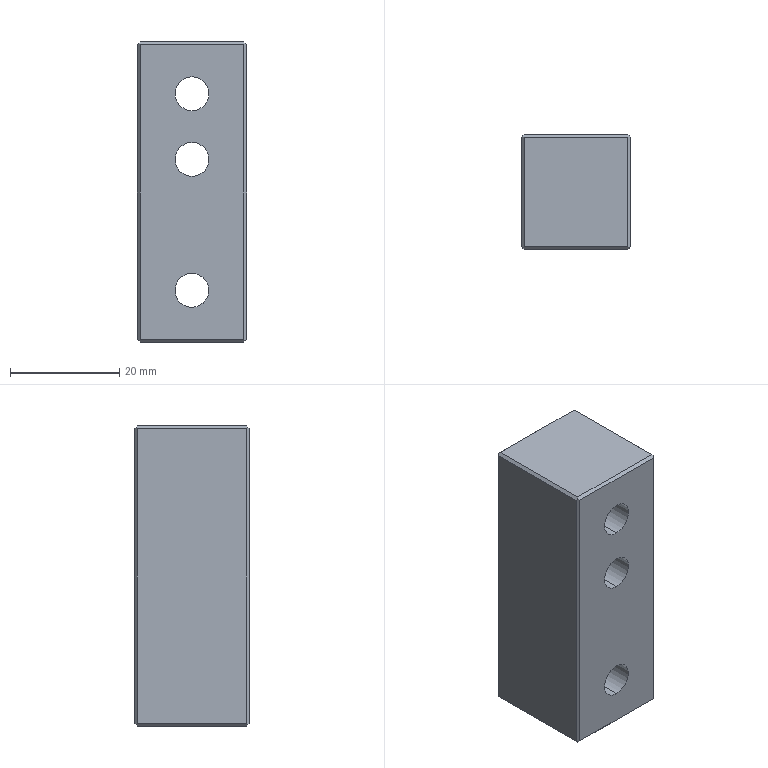Part | NX | features BREP 1 | 1 solid | 33 faces | box 20 x 21 x 55 mm | volume 20710 mm3 | plane 19 | cylinder 8 | cone 6 | commonest cylinder face diameters 6.2 x6 9.5 x2
STEP:
#1=CARTESIAN_POINT('',(0.,20.5,7.25));
#2=VERTEX_POINT('',#1);
#3=CARTESIAN_POINT('',(0.,20.5,16.75));
#4=VERTEX_POINT('',#3);
#5=CARTESIAN_POINT('',(0.,20.5,12.));
#6=DIRECTION('',(0.,1.,0.));
#7=DIRECTION('',(0.,0.,1.));
#8=AXIS2_PLACEMENT_3D('',#5,#6,#7);
#9=CIRCLE('',#8,4.75);
#10=EDGE_CURVE('',#2,#4,#9,.T.);
#11=ORIENTED_EDGE('',*,*,#10,.F.);
#12=CARTESIAN_POINT('',(0.,21.,6.75));
#13=VERTEX_POINT('',#12);
#14=CARTESIAN_POINT('',(0.,21.,6.75));
#15=DIRECTION('',(0.,0.7071,-0.7071));
#16=VECTOR('',#15,1000.);
#17=LINE('',#14,#16);
#18=EDGE_CURVE('',#2,#13,#17,.T.);
#19=ORIENTED_EDGE('',*,*,#18,.T.);
#20=CARTESIAN_POINT('',(0.,21.,17.25));
#21=VERTEX_POINT('',#20);
#22=CARTESIAN_POINT('',(0.,21.,12.));
#23=DIRECTION('',(0.,-1.,0.));
#24=DIRECTION('',(0.,0.,1.));
#25=AXIS2_PLACEMENT_3D('',#22,#23,#24);
#26=CIRCLE('',#25,5.25);
#27=EDGE_CURVE('',#21,#13,#26,.T.);
#28=ORIENTED_EDGE('',*,*,#27,.F.);
#29=CARTESIAN_POINT('',(0.,21.,17.25));
#30=DIRECTION('',(0.,0.7071,0.7071));
#31=VECTOR('',#30,1000.);
#32=LINE('',#29,#31);
#33=EDGE_CURVE('',#4,#21,#32,.T.);
#34=ORIENTED_EDGE('',*,*,#33,.F.);
#35=EDGE_LOOP('',(#11,#19,#28,#34));
#36=FACE_BOUND('',#35,.T.);
#37=CARTESIAN_POINT('',(0.,21.,12.));
#38=DIRECTION('',(0.,1.,0.));
#39=DIRECTION('',(0.,0.,-1.));
#40=AXIS2_PLACEMENT_3D('',#37,#38,#39);
#41=CONICAL_SURFACE('',#40,5.25,0.7854);
#42=ADVANCED_FACE('',(#36),#41,.F.);
#43=CARTESIAN_POINT('',(-0.02287,20.5,-27.126));
#44=VERTEX_POINT('',#43);
#45=CARTESIAN_POINT('',(-0.02287,20.5,-20.926));
#46=VERTEX_POINT('',#45);
#47=CARTESIAN_POINT('',(-0.02287,20.5,-24.026));
#48=DIRECTION('',(0.,1.,0.));
#49=DIRECTION('',(0.,0.,1.));
#50=AXIS2_PLACEMENT_3D('',#47,#48,#49);
#51=CIRCLE('',#50,3.1);
#52=EDGE_CURVE('',#44,#46,#51,.T.);
#53=ORIENTED_EDGE('',*,*,#52,.F.);
#54=CARTESIAN_POINT('',(-0.02287,21.,-27.626));
#55=VERTEX_POINT('',#54);
#56=CARTESIAN_POINT('',(-0.02287,21.,-27.626));
#57=DIRECTION('',(0.,0.7071,-0.7071));
#58=VECTOR('',#57,1000.);
#59=LINE('',#56,#58);
#60=EDGE_CURVE('',#44,#55,#59,.T.);
#61=ORIENTED_EDGE('',*,*,#60,.T.);
#62=CARTESIAN_POINT('',(-0.02287,21.,-20.426));
#63=VERTEX_POINT('',#62);
#64=CARTESIAN_POINT('',(-0.02287,21.,-24.026));
#65=DIRECTION('',(0.,-1.,0.));
#66=DIRECTION('',(0.,0.,1.));
#67=AXIS2_PLACEMENT_3D('',#64,#65,#66);
#68=CIRCLE('',#67,3.6);
#69=EDGE_CURVE('',#63,#55,#68,.T.);
#70=ORIENTED_EDGE('',*,*,#69,.F.);
#71=CARTESIAN_POINT('',(-0.02287,21.,-20.426));
#72=DIRECTION('',(0.,0.7071,0.7071));
#73=VECTOR('',#72,1000.);
#74=LINE('',#71,#73);
#75=EDGE_CURVE('',#46,#63,#74,.T.);
#76=ORIENTED_EDGE('',*,*,#75,.F.);
#77=EDGE_LOOP('',(#53,#61,#70,#76));
#78=FACE_BOUND('',#77,.T.);
#79=CARTESIAN_POINT('',(-0.02287,21.,-24.026));
#80=DIRECTION('',(0.,1.,0.));
#81=DIRECTION('',(0.,0.,-1.));
#82=AXIS2_PLACEMENT_3D('',#79,#80,#81);
#83=CONICAL_SURFACE('',#82,3.6,0.7854);
#84=ADVANCED_FACE('',(#78),#83,.F.);
#85=CARTESIAN_POINT('',(0.,20.5,-3.126));
#86=VERTEX_POINT('',#85);
#87=CARTESIAN_POINT('',(0.,20.5,3.074));
#88=VERTEX_POINT('',#87);
#89=CARTESIAN_POINT('',(0.,20.5,-0.02589));
#90=DIRECTION('',(0.,1.,0.));
#91=DIRECTION('',(0.,0.,1.));
#92=AXIS2_PLACEMENT_3D('',#89,#90,#91);
#93=CIRCLE('',#92,3.1);
#94=EDGE_CURVE('',#86,#88,#93,.T.);
#95=ORIENTED_EDGE('',*,*,#94,.F.);
#96=CARTESIAN_POINT('',(0.,21.,-3.626));
#97=VERTEX_POINT('',#96);
#98=CARTESIAN_POINT('',(0.,21.,-3.626));
#99=DIRECTION('',(0.,0.7071,-0.7071));
#100=VECTOR('',#99,1000.);
#101=LINE('',#98,#100);
#102=EDGE_CURVE('',#86,#97,#101,.T.);
#103=ORIENTED_EDGE('',*,*,#102,.T.);
#104=CARTESIAN_POINT('',(0.,21.,3.574));
#105=VERTEX_POINT('',#104);
#106=CARTESIAN_POINT('',(0.,21.,-0.02589));
#107=DIRECTION('',(0.,-1.,0.));
#108=DIRECTION('',(0.,0.,1.));
#109=AXIS2_PLACEMENT_3D('',#106,#107,#108);
#110=CIRCLE('',#109,3.6);
#111=EDGE_CURVE('',#105,#97,#110,.T.);
#112=ORIENTED_EDGE('',*,*,#111,.F.);
#113=CARTESIAN_POINT('',(0.,21.,3.574));
#114=DIRECTION('',(0.,0.7071,0.7071));
#115=VECTOR('',#114,1000.);
#116=LINE('',#113,#115);
#117=EDGE_CURVE('',#88,#105,#116,.T.);
#118=ORIENTED_EDGE('',*,*,#117,.F.);
#119=EDGE_LOOP('',(#95,#103,#112,#118));
#120=FACE_BOUND('',#119,.T.);
#121=CARTESIAN_POINT('',(0.,21.,-0.02589));
#122=DIRECTION('',(0.,1.,0.));
#123=DIRECTION('',(0.,0.,-1.));
#124=AXIS2_PLACEMENT_3D('',#121,#122,#123);
#125=CONICAL_SURFACE('',#124,3.6,0.7854);
#126=ADVANCED_FACE('',(#120),#125,.F.);
#127=CARTESIAN_POINT('',(-0.02287,0.,-20.926));
#128=VERTEX_POINT('',#127);
#129=CARTESIAN_POINT('',(-0.02287,0.,-27.126));
#130=VERTEX_POINT('',#129);
#131=CARTESIAN_POINT('',(-0.02287,0.,-24.026));
#132=DIRECTION('',(0.,-1.,0.));
#133=DIRECTION('',(0.,0.,1.));
#134=AXIS2_PLACEMENT_3D('',#131,#132,#133);
#135=CIRCLE('',#134,3.1);
#136=EDGE_CURVE('',#128,#130,#135,.T.);
#137=ORIENTED_EDGE('',*,*,#136,.T.);
#138=CARTESIAN_POINT('',(-0.02287,21.,-27.126));
#139=DIRECTION('',(0.,1.,0.));
#140=VECTOR('',#139,1000.);
#141=LINE('',#138,#140);
#142=EDGE_CURVE('',#130,#44,#141,.T.);
#143=ORIENTED_EDGE('',*,*,#142,.T.);
#144=ORIENTED_EDGE('',*,*,#52,.T.);
#145=CARTESIAN_POINT('',(-0.02287,21.,-20.926));
#146=DIRECTION('',(0.,1.,0.));
#147=VECTOR('',#146,1000.);
#148=LINE('',#145,#147);
#149=EDGE_CURVE('',#128,#46,#148,.T.);
#150=ORIENTED_EDGE('',*,*,#149,.F.);
#151=EDGE_LOOP('',(#137,#143,#144,#150));
#152=FACE_BOUND('',#151,.T.);
#153=CARTESIAN_POINT('',(-0.02287,21.,-24.026));
#154=DIRECTION('',(0.,1.,0.));
#155=DIRECTION('',(0.,0.,-1.));
#156=AXIS2_PLACEMENT_3D('',#153,#154,#155);
#157=CYLINDRICAL_SURFACE('',#156,3.1);
#158=ADVANCED_FACE('',(#152),#157,.F.);
#159=CARTESIAN_POINT('',(0.,0.,15.1));
#160=VERTEX_POINT('',#159);
#161=CARTESIAN_POINT('',(0.,0.,8.9));
#162=VERTEX_POINT('',#161);
#163=CARTESIAN_POINT('',(0.,0.,12.));
#164=DIRECTION('',(0.,-1.,0.));
#165=DIRECTION('',(0.,0.,1.));
#166=AXIS2_PLACEMENT_3D('',#163,#164,#165);
#167=CIRCLE('',#166,3.1);
#168=EDGE_CURVE('',#160,#162,#167,.T.);
#169=ORIENTED_EDGE('',*,*,#168,.T.);
#170=CARTESIAN_POINT('',(0.,10.4,8.9));
#171=VERTEX_POINT('',#170);
#172=CARTESIAN_POINT('',(0.,21.,8.9));
#173=DIRECTION('',(0.,1.,0.));
#174=VECTOR('',#173,1000.);
#175=LINE('',#172,#174);
#176=EDGE_CURVE('',#162,#171,#175,.T.);
#177=ORIENTED_EDGE('',*,*,#176,.T.);
#178=CARTESIAN_POINT('',(0.,10.4,15.1));
#179=VERTEX_POINT('',#178);
#180=CARTESIAN_POINT('',(0.,10.4,12.));
#181=DIRECTION('',(0.,-1.,0.));
#182=DIRECTION('',(0.,0.,1.));
#183=AXIS2_PLACEMENT_3D('',#180,#181,#182);
#184=CIRCLE('',#183,3.1);
#185=EDGE_CURVE('',#179,#171,#184,.T.);
#186=ORIENTED_EDGE('',*,*,#185,.F.);
#187=CARTESIAN_POINT('',(0.,21.,15.1));
#188=DIRECTION('',(0.,1.,0.));
#189=VECTOR('',#188,1000.);
#190=LINE('',#187,#189);
#191=EDGE_CURVE('',#160,#179,#190,.T.);
#192=ORIENTED_EDGE('',*,*,#191,.F.);
#193=EDGE_LOOP('',(#169,#177,#186,#192));
#194=FACE_BOUND('',#193,.T.);
#195=CARTESIAN_POINT('',(0.,21.,12.));
#196=DIRECTION('',(0.,1.,0.));
#197=DIRECTION('',(0.,0.,-1.));
#198=AXIS2_PLACEMENT_3D('',#195,#196,#197);
#199=CYLINDRICAL_SURFACE('',#198,3.1);
#200=ADVANCED_FACE('',(#194),#199,.F.);
#201=CARTESIAN_POINT('',(0.,0.,3.074));
#202=VERTEX_POINT('',#201);
#203=CARTESIAN_POINT('',(0.,0.,-3.126));
#204=VERTEX_POINT('',#203);
#205=CARTESIAN_POINT('',(0.,0.,-0.02589));
#206=DIRECTION('',(0.,-1.,0.));
#207=DIRECTION('',(0.,0.,1.));
#208=AXIS2_PLACEMENT_3D('',#205,#206,#207);
#209=CIRCLE('',#208,3.1);
#210=EDGE_CURVE('',#202,#204,#209,.T.);
#211=ORIENTED_EDGE('',*,*,#210,.T.);
#212=CARTESIAN_POINT('',(0.,21.,-3.126));
#213=DIRECTION('',(0.,1.,0.));
#214=VECTOR('',#213,1000.);
#215=LINE('',#212,#214);
#216=EDGE_CURVE('',#204,#86,#215,.T.);
#217=ORIENTED_EDGE('',*,*,#216,.T.);
#218=ORIENTED_EDGE('',*,*,#94,.T.);
#219=CARTESIAN_POINT('',(0.,21.,3.074));
#220=DIRECTION('',(0.,1.,0.));
#221=VECTOR('',#220,1000.);
#222=LINE('',#219,#221);
#223=EDGE_CURVE('',#202,#88,#222,.T.);
#224=ORIENTED_EDGE('',*,*,#223,.F.);
#225=EDGE_LOOP('',(#211,#217,#218,#224));
#226=FACE_BOUND('',#225,.T.);
#227=CARTESIAN_POINT('',(0.,21.,-0.02589));
#228=DIRECTION('',(0.,1.,0.));
#229=DIRECTION('',(0.,0.,-1.));
#230=AXIS2_PLACEMENT_3D('',#227,#228,#229);
#231=CYLINDRICAL_SURFACE('',#230,3.1);
#232=ADVANCED_FACE('',(#226),#231,.F.);
#233=CARTESIAN_POINT('',(0.,10.4,7.25));
#234=VERTEX_POINT('',#233);
#235=CARTESIAN_POINT('',(0.,10.4,16.75));
#236=VERTEX_POINT('',#235);
#237=CARTESIAN_POINT('',(0.,10.4,12.));
#238=DIRECTION('',(0.,1.,0.));
#239=DIRECTION('',(0.,0.,1.));
#240=AXIS2_PLACEMENT_3D('',#237,#238,#239);
#241=CIRCLE('',#240,4.75);
#242=EDGE_CURVE('',#234,#236,#241,.T.);
#243=ORIENTED_EDGE('',*,*,#242,.F.);
#244=CARTESIAN_POINT('',(0.,21.,7.25));
#245=DIRECTION('',(0.,1.,0.));
#246=VECTOR('',#245,1000.);
#247=LINE('',#244,#246);
#248=EDGE_CURVE('',#234,#2,#247,.T.);
#249=ORIENTED_EDGE('',*,*,#248,.T.);
#250=ORIENTED_EDGE('',*,*,#10,.T.);
#251=CARTESIAN_POINT('',(0.,21.,16.75));
#252=DIRECTION('',(0.,1.,0.));
#253=VECTOR('',#252,1000.);
#254=LINE('',#251,#253);
#255=EDGE_CURVE('',#236,#4,#254,.T.);
#256=ORIENTED_EDGE('',*,*,#255,.F.);
#257=EDGE_LOOP('',(#243,#249,#250,#256));
#258=FACE_BOUND('',#257,.T.);
#259=CARTESIAN_POINT('',(0.,21.,12.));
#260=DIRECTION('',(0.,1.,0.));
#261=DIRECTION('',(0.,0.,-1.));
#262=AXIS2_PLACEMENT_3D('',#259,#260,#261);
#263=CYLINDRICAL_SURFACE('',#262,4.75);
#264=ADVANCED_FACE('',(#258),#263,.F.);
#265=CARTESIAN_POINT('',(10.,0.5,-33.));
#266=VERTEX_POINT('',#265);
#267=CARTESIAN_POINT('',(10.,20.5,-33.));
#268=VERTEX_POINT('',#267);
#269=CARTESIAN_POINT('',(10.,0.,-33.));
#270=DIRECTION('',(0.,1.,0.));
#271=VECTOR('',#270,1000.);
#272=LINE('',#269,#271);
#273=EDGE_CURVE('',#266,#268,#272,.T.);
#274=ORIENTED_EDGE('',*,*,#273,.T.);
#275=CARTESIAN_POINT('',(10.,20.5,21.));
#276=VERTEX_POINT('',#275);
#277=CARTESIAN_POINT('',(10.,20.5,36.5));
#278=DIRECTION('',(0.,0.,1.));
#279=VECTOR('',#278,1000.);
#280=LINE('',#277,#279);
#281=EDGE_CURVE('',#268,#276,#280,.T.);
#282=ORIENTED_EDGE('',*,*,#281,.T.);
#283=CARTESIAN_POINT('',(10.,0.5,21.));
#284=VERTEX_POINT('',#283);
#285=CARTESIAN_POINT('',(10.,0.,21.));
#286=DIRECTION('',(0.,-1.,0.));
#287=VECTOR('',#286,1000.);
#288=LINE('',#285,#287);
#289=EDGE_CURVE('',#276,#284,#288,.T.);
#290=ORIENTED_EDGE('',*,*,#289,.T.);
#291=CARTESIAN_POINT('',(10.,0.5,36.5));
#292=DIRECTION('',(0.,0.,-1.));
#293=VECTOR('',#292,1000.);
#294=LINE('',#291,#293);
#295=EDGE_CURVE('',#284,#266,#294,.T.);
#296=ORIENTED_EDGE('',*,*,#295,.T.);
#297=EDGE_LOOP('',(#274,#282,#290,#296));
#298=FACE_BOUND('',#297,.T.);
#299=CARTESIAN_POINT('',(10.,0.,36.5));
#300=DIRECTION('',(1.,0.,0.));
#301=DIRECTION('',(0.,0.,1.));
#302=AXIS2_PLACEMENT_3D('',#299,#300,#301);
#303=PLANE('',#302);
#304=ADVANCED_FACE('',(#298),#303,.T.);
#305=CARTESIAN_POINT('',(9.5,21.,-33.));
#306=VERTEX_POINT('',#305);
#307=CARTESIAN_POINT('',(9.5,21.,21.));
#308=VERTEX_POINT('',#307);
#309=CARTESIAN_POINT('',(9.5,21.,-6.));
#310=DIRECTION('',(0.,0.,1.));
#311=VECTOR('',#310,1000.);
#312=LINE('',#309,#311);
#313=EDGE_CURVE('',#306,#308,#312,.T.);
#314=ORIENTED_EDGE('',*,*,#313,.T.);
#315=CARTESIAN_POINT('',(9.75,20.75,21.25));
#316=VERTEX_POINT('',#315);
#317=CARTESIAN_POINT('',(9.75,20.75,21.25));
#318=DIRECTION('',(-0.5774,0.5774,-0.5774));
#319=VECTOR('',#318,1000.);
#320=LINE('',#317,#319);
#321=EDGE_CURVE('',#316,#308,#320,.T.);
#322=ORIENTED_EDGE('',*,*,#321,.F.);
#323=CARTESIAN_POINT('',(9.75,20.75,21.25));
#324=DIRECTION('',(0.5774,-0.5774,-0.5774));
#325=VECTOR('',#324,1000.);
#326=LINE('',#323,#325);
#327=EDGE_CURVE('',#316,#276,#326,.T.);
#328=ORIENTED_EDGE('',*,*,#327,.T.);
#329=ORIENTED_EDGE('',*,*,#281,.F.);
#330=CARTESIAN_POINT('',(9.75,20.75,-33.25));
#331=VERTEX_POINT('',#330);
#332=CARTESIAN_POINT('',(10.,20.5,-33.));
#333=DIRECTION('',(-0.5774,0.5774,-0.5774));
#334=VECTOR('',#333,1000.);
#335=LINE('',#332,#334);
#336=EDGE_CURVE('',#268,#331,#335,.T.);
#337=ORIENTED_EDGE('',*,*,#336,.T.);
#338=CARTESIAN_POINT('',(9.5,21.,-33.));
#339=DIRECTION('',(0.5774,-0.5774,-0.5774));
#340=VECTOR('',#339,1000.);
#341=LINE('',#338,#340);
#342=EDGE_CURVE('',#306,#331,#341,.T.);
#343=ORIENTED_EDGE('',*,*,#342,.F.);
#344=EDGE_LOOP('',(#314,#322,#328,#329,#337,#343));
#345=FACE_BOUND('',#344,.T.);
#346=CARTESIAN_POINT('',(9.75,20.75,-6.));
#347=DIRECTION('',(0.7071,0.7071,0.));
#348=DIRECTION('',(0.7071,-0.7071,0.));
#349=AXIS2_PLACEMENT_3D('',#346,#347,#348);
#350=PLANE('',#349);
#351=ADVANCED_FACE('',(#345),#350,.T.);
#352=ORIENTED_EDGE('',*,*,#273,.F.);
#353=CARTESIAN_POINT('',(9.75,0.25,-33.25));
#354=VERTEX_POINT('',#353);
#355=CARTESIAN_POINT('',(10.,0.5,-33.));
#356=DIRECTION('',(-0.5774,-0.5774,-0.5774));
#357=VECTOR('',#356,1000.);
#358=LINE('',#355,#357);
#359=EDGE_CURVE('',#266,#354,#358,.T.);
#360=ORIENTED_EDGE('',*,*,#359,.T.);
#361=CARTESIAN_POINT('',(9.5,0.5,-33.5));
#362=VERTEX_POINT('',#361);
#363=CARTESIAN_POINT('',(9.5,0.5,-33.5));
#364=DIRECTION('',(0.5774,-0.5774,0.5774));
#365=VECTOR('',#364,1000.);
#366=LINE('',#363,#365);
#367=EDGE_CURVE('',#362,#354,#366,.T.);
#368=ORIENTED_EDGE('',*,*,#367,.F.);
#369=CARTESIAN_POINT('',(9.5,20.5,-33.5));
#370=VERTEX_POINT('',#369);
#371=CARTESIAN_POINT('',(9.5,10.5,-33.5));
#372=DIRECTION('',(0.,1.,0.));
#373=VECTOR('',#372,1000.);
#374=LINE('',#371,#373);
#375=EDGE_CURVE('',#362,#370,#374,.T.);
#376=ORIENTED_EDGE('',*,*,#375,.T.);
#377=CARTESIAN_POINT('',(9.75,20.75,-33.25));
#378=DIRECTION('',(-0.5774,-0.5774,-0.5774));
#379=VECTOR('',#378,1000.);
#380=LINE('',#377,#379);
#381=EDGE_CURVE('',#331,#370,#380,.T.);
#382=ORIENTED_EDGE('',*,*,#381,.F.);
#383=ORIENTED_EDGE('',*,*,#336,.F.);
#384=EDGE_LOOP('',(#352,#360,#368,#376,#382,#383));
#385=FACE_BOUND('',#384,.T.);
#386=CARTESIAN_POINT('',(9.75,10.5,-33.25));
#387=DIRECTION('',(0.7071,0.,-0.7071));
#388=DIRECTION('',(0.7071,0.,0.7071));
#389=AXIS2_PLACEMENT_3D('',#386,#387,#388);
#390=PLANE('',#389);
#391=ADVANCED_FACE('',(#385),#390,.T.);
#392=ORIENTED_EDGE('',*,*,#295,.F.);
#393=CARTESIAN_POINT('',(9.75,0.25,21.25));
#394=VERTEX_POINT('',#393);
#395=CARTESIAN_POINT('',(10.,0.5,21.));
#396=DIRECTION('',(-0.5774,-0.5774,0.5774));
#397=VECTOR('',#396,1000.);
#398=LINE('',#395,#397);
#399=EDGE_CURVE('',#284,#394,#398,.T.);
#400=ORIENTED_EDGE('',*,*,#399,.T.);
#401=CARTESIAN_POINT('',(9.5,0.,21.));
#402=VERTEX_POINT('',#401);
#403=CARTESIAN_POINT('',(9.5,0.,21.));
#404=DIRECTION('',(0.5774,0.5774,0.5774));
#405=VECTOR('',#404,1000.);
#406=LINE('',#403,#405);
#407=EDGE_CURVE('',#402,#394,#406,.T.);
#408=ORIENTED_EDGE('',*,*,#407,.F.);
#409=CARTESIAN_POINT('',(9.5,0.,-33.));
#410=VERTEX_POINT('',#409);
#411=CARTESIAN_POINT('',(9.5,0.,-6.));
#412=DIRECTION('',(0.,0.,-1.));
#413=VECTOR('',#412,1000.);
#414=LINE('',#411,#413);
#415=EDGE_CURVE('',#402,#410,#414,.T.);
#416=ORIENTED_EDGE('',*,*,#415,.T.);
#417=CARTESIAN_POINT('',(9.75,0.25,-33.25));
#418=DIRECTION('',(-0.5774,-0.5774,0.5774));
#419=VECTOR('',#418,1000.);
#420=LINE('',#417,#419);
#421=EDGE_CURVE('',#354,#410,#420,.T.);
#422=ORIENTED_EDGE('',*,*,#421,.F.);
#423=ORIENTED_EDGE('',*,*,#359,.F.);
#424=EDGE_LOOP('',(#392,#400,#408,#416,#422,#423));
#425=FACE_BOUND('',#424,.T.);
#426=CARTESIAN_POINT('',(9.75,0.25,-6.));
#427=DIRECTION('',(0.7071,-0.7071,0.));
#428=DIRECTION('',(-0.7071,-0.7071,0.));
#429=AXIS2_PLACEMENT_3D('',#426,#427,#428);
#430=PLANE('',#429);
#431=ADVANCED_FACE('',(#425),#430,.T.);
#432=CARTESIAN_POINT('',(9.5,20.5,21.5));
#433=VERTEX_POINT('',#432);
#434=CARTESIAN_POINT('',(9.5,0.5,21.5));
#435=VERTEX_POINT('',#434);
#436=CARTESIAN_POINT('',(9.5,10.5,21.5));
#437=DIRECTION('',(0.,-1.,0.));
#438=VECTOR('',#437,1000.);
#439=LINE('',#436,#438);
#440=EDGE_CURVE('',#433,#435,#439,.T.);
#441=ORIENTED_EDGE('',*,*,#440,.T.);
#442=CARTESIAN_POINT('',(9.75,0.25,21.25));
#443=DIRECTION('',(-0.5774,0.5774,0.5774));
#444=VECTOR('',#443,1000.);
#445=LINE('',#442,#444);
#446=EDGE_CURVE('',#394,#435,#445,.T.);
#447=ORIENTED_EDGE('',*,*,#446,.F.);
#448=ORIENTED_EDGE('',*,*,#399,.F.);
#449=ORIENTED_EDGE('',*,*,#289,.F.);
#450=ORIENTED_EDGE('',*,*,#327,.F.);
#451=CARTESIAN_POINT('',(9.5,20.5,21.5));
#452=DIRECTION('',(0.5774,0.5774,-0.5774));
#453=VECTOR('',#452,1000.);
#454=LINE('',#451,#453);
#455=EDGE_CURVE('',#433,#316,#454,.T.);
#456=ORIENTED_EDGE('',*,*,#455,.F.);
#457=EDGE_LOOP('',(#441,#447,#448,#449,#450,#456));
#458=FACE_BOUND('',#457,.T.);
#459=CARTESIAN_POINT('',(9.75,10.5,21.25));
#460=DIRECTION('',(0.7071,0.,0.7071));
#461=DIRECTION('',(-0.7071,0.,0.7071));
#462=AXIS2_PLACEMENT_3D('',#459,#460,#461);
#463=PLANE('',#462);
#464=ADVANCED_FACE('',(#458),#463,.T.);
#465=CARTESIAN_POINT('',(-9.5,21.,21.));
#466=VERTEX_POINT('',#465);
#467=CARTESIAN_POINT('',(0.,21.,21.));
#468=DIRECTION('',(1.,0.,0.));
#469=VECTOR('',#468,1000.);
#470=LINE('',#467,#469);
#471=EDGE_CURVE('',#466,#308,#470,.T.);
#472=ORIENTED_EDGE('',*,*,#471,.T.);
#473=ORIENTED_EDGE('',*,*,#313,.F.);
#474=CARTESIAN_POINT('',(-9.5,21.,-33.));
#475=VERTEX_POINT('',#474);
#476=CARTESIAN_POINT('',(0.,21.,-33.));
#477=DIRECTION('',(-1.,0.,0.));
#478=VECTOR('',#477,1000.);
#479=LINE('',#476,#478);
#480=EDGE_CURVE('',#306,#475,#479,.T.);
#481=ORIENTED_EDGE('',*,*,#480,.T.);
#482=CARTESIAN_POINT('',(-9.5,21.,0.));
#483=DIRECTION('',(0.,0.,1.));
#484=VECTOR('',#483,1000.);
#485=LINE('',#482,#484);
#486=EDGE_CURVE('',#475,#466,#485,.T.);
#487=ORIENTED_EDGE('',*,*,#486,.T.);
#488=EDGE_LOOP('',(#472,#473,#481,#487));
#489=FACE_BOUND('',#488,.T.);
#490=ORIENTED_EDGE('',*,*,#27,.T.);
#491=CARTESIAN_POINT('',(0.,21.,12.));
#492=DIRECTION('',(0.,-1.,0.));
#493=DIRECTION('',(0.,0.,1.));
#494=AXIS2_PLACEMENT_3D('',#491,#492,#493);
#495=CIRCLE('',#494,5.25);
#496=EDGE_CURVE('',#13,#21,#495,.T.);
#497=ORIENTED_EDGE('',*,*,#496,.T.);
#498=EDGE_LOOP('',(#490,#497));
#499=FACE_BOUND('',#498,.T.);
#500=ORIENTED_EDGE('',*,*,#69,.T.);
#501=CARTESIAN_POINT('',(-0.02287,21.,-24.026));
#502=DIRECTION('',(0.,-1.,0.));
#503=DIRECTION('',(0.,0.,1.));
#504=AXIS2_PLACEMENT_3D('',#501,#502,#503);
#505=CIRCLE('',#504,3.6);
#506=EDGE_CURVE('',#55,#63,#505,.T.);
#507=ORIENTED_EDGE('',*,*,#506,.T.);
#508=EDGE_LOOP('',(#500,#507));
#509=FACE_BOUND('',#508,.T.);
#510=ORIENTED_EDGE('',*,*,#111,.T.);
#511=CARTESIAN_POINT('',(0.,21.,-0.02589));
#512=DIRECTION('',(0.,-1.,0.));
#513=DIRECTION('',(0.,0.,1.));
#514=AXIS2_PLACEMENT_3D('',#511,#512,#513);
#515=CIRCLE('',#514,3.6);
#516=EDGE_CURVE('',#97,#105,#515,.T.);
#517=ORIENTED_EDGE('',*,*,#516,.T.);
#518=EDGE_LOOP('',(#510,#517));
#519=FACE_BOUND('',#518,.T.);
#520=CARTESIAN_POINT('',(0.,21.,0.));
#521=DIRECTION('',(0.,1.,0.));
#522=DIRECTION('',(0.,0.,-1.));
#523=AXIS2_PLACEMENT_3D('',#520,#521,#522);
#524=PLANE('',#523);
#525=ADVANCED_FACE('',(#489,#499,#509,#519),#524,.T.);
#526=ORIENTED_EDGE('',*,*,#375,.F.);
#527=CARTESIAN_POINT('',(-9.5,0.5,-33.5));
#528=VERTEX_POINT('',#527);
#529=CARTESIAN_POINT('',(10.,0.5,-33.5));
#530=DIRECTION('',(-1.,0.,0.));
#531=VECTOR('',#530,1000.);
#532=LINE('',#529,#531);
#533=EDGE_CURVE('',#362,#528,#532,.T.);
#534=ORIENTED_EDGE('',*,*,#533,.T.);
#535=CARTESIAN_POINT('',(-9.5,20.5,-33.5));
#536=VERTEX_POINT('',#535);
#537=CARTESIAN_POINT('',(-9.5,0.,-33.5));
#538=DIRECTION('',(0.,1.,0.));
#539=VECTOR('',#538,1000.);
#540=LINE('',#537,#539);
#541=EDGE_CURVE('',#528,#536,#540,.T.);
#542=ORIENTED_EDGE('',*,*,#541,.T.);
#543=CARTESIAN_POINT('',(10.,20.5,-33.5));
#544=DIRECTION('',(1.,0.,0.));
#545=VECTOR('',#544,1000.);
#546=LINE('',#543,#545);
#547=EDGE_CURVE('',#536,#370,#546,.T.);
#548=ORIENTED_EDGE('',*,*,#547,.T.);
#549=EDGE_LOOP('',(#526,#534,#542,#548));
#550=FACE_BOUND('',#549,.T.);
#551=CARTESIAN_POINT('',(10.,0.,-33.5));
#552=DIRECTION('',(0.,0.,-1.));
#553=DIRECTION('',(1.,0.,0.));
#554=AXIS2_PLACEMENT_3D('',#551,#552,#553);
#555=PLANE('',#554);
#556=ADVANCED_FACE('',(#550),#555,.T.);
#557=CARTESIAN_POINT('',(-9.5,0.,-33.));
#558=VERTEX_POINT('',#557);
#559=CARTESIAN_POINT('',(0.,0.,-33.));
#560=DIRECTION('',(-1.,0.,0.));
#561=VECTOR('',#560,1000.);
#562=LINE('',#559,#561);
#563=EDGE_CURVE('',#410,#558,#562,.T.);
#564=ORIENTED_EDGE('',*,*,#563,.F.);
#565=ORIENTED_EDGE('',*,*,#415,.F.);
#566=CARTESIAN_POINT('',(-9.5,0.,21.));
#567=VERTEX_POINT('',#566);
#568=CARTESIAN_POINT('',(0.,0.,21.));
#569=DIRECTION('',(1.,0.,0.));
#570=VECTOR('',#569,1000.);
#571=LINE('',#568,#570);
#572=EDGE_CURVE('',#567,#402,#571,.T.);
#573=ORIENTED_EDGE('',*,*,#572,.F.);
#574=CARTESIAN_POINT('',(-9.5,0.,0.));
#575=DIRECTION('',(0.,0.,1.));
#576=VECTOR('',#575,1000.);
#577=LINE('',#574,#576);
#578=EDGE_CURVE('',#558,#567,#577,.T.);
#579=ORIENTED_EDGE('',*,*,#578,.F.);
#580=EDGE_LOOP('',(#564,#565,#573,#579));
#581=FACE_BOUND('',#580,.T.);
#582=ORIENTED_EDGE('',*,*,#136,.F.);
#583=CARTESIAN_POINT('',(-0.02287,0.,-24.026));
#584=DIRECTION('',(0.,-1.,0.));
#585=DIRECTION('',(0.,0.,1.));
#586=AXIS2_PLACEMENT_3D('',#583,#584,#585);
#587=CIRCLE('',#586,3.1);
#588=EDGE_CURVE('',#130,#128,#587,.T.);
#589=ORIENTED_EDGE('',*,*,#588,.F.);
#590=EDGE_LOOP('',(#582,#589));
#591=FACE_BOUND('',#590,.T.);
#592=ORIENTED_EDGE('',*,*,#168,.F.);
#593=CARTESIAN_POINT('',(0.,0.,12.));
#594=DIRECTION('',(0.,-1.,0.));
#595=DIRECTION('',(0.,0.,1.));
#596=AXIS2_PLACEMENT_3D('',#593,#594,#595);
#597=CIRCLE('',#596,3.1);
#598=EDGE_CURVE('',#162,#160,#597,.T.);
#599=ORIENTED_EDGE('',*,*,#598,.F.);
#600=EDGE_LOOP('',(#592,#599));
#601=FACE_BOUND('',#600,.T.);
#602=ORIENTED_EDGE('',*,*,#210,.F.);
#603=CARTESIAN_POINT('',(0.,0.,-0.02589));
#604=DIRECTION('',(0.,-1.,0.));
#605=DIRECTION('',(0.,0.,1.));
#606=AXIS2_PLACEMENT_3D('',#603,#604,#605);
#607=CIRCLE('',#606,3.1);
#608=EDGE_CURVE('',#204,#202,#607,.T.);
#609=ORIENTED_EDGE('',*,*,#608,.F.);
#610=EDGE_LOOP('',(#602,#609));
#611=FACE_BOUND('',#610,.T.);
#612=CARTESIAN_POINT('',(0.,0.,0.));
#613=DIRECTION('',(0.,1.,0.));
#614=DIRECTION('',(0.,0.,-1.));
#615=AXIS2_PLACEMENT_3D('',#612,#613,#614);
#616=PLANE('',#615);
#617=ADVANCED_FACE('',(#581,#591,#601,#611),#616,.F.);
#618=CARTESIAN_POINT('',(-9.5,20.5,21.5));
#619=VERTEX_POINT('',#618);
#620=CARTESIAN_POINT('',(-10.,20.5,21.5));
#621=DIRECTION('',(-1.,0.,0.));
#622=VECTOR('',#621,1000.);
#623=LINE('',#620,#622);
#624=EDGE_CURVE('',#433,#619,#623,.T.);
#625=ORIENTED_EDGE('',*,*,#624,.T.);
#626=CARTESIAN_POINT('',(-9.5,0.5,21.5));
#627=VERTEX_POINT('',#626);
#628=CARTESIAN_POINT('',(-9.5,0.,21.5));
#629=DIRECTION('',(0.,-1.,0.));
#630=VECTOR('',#629,1000.);
#631=LINE('',#628,#630);
#632=EDGE_CURVE('',#619,#627,#631,.T.);
#633=ORIENTED_EDGE('',*,*,#632,.T.);
#634=CARTESIAN_POINT('',(-10.,0.5,21.5));
#635=DIRECTION('',(1.,0.,0.));
#636=VECTOR('',#635,1000.);
#637=LINE('',#634,#636);
#638=EDGE_CURVE('',#627,#435,#637,.T.);
#639=ORIENTED_EDGE('',*,*,#638,.T.);
#640=ORIENTED_EDGE('',*,*,#440,.F.);
#641=EDGE_LOOP('',(#625,#633,#639,#640));
#642=FACE_BOUND('',#641,.T.);
#643=CARTESIAN_POINT('',(-10.,0.,21.5));
#644=DIRECTION('',(0.,0.,1.));
#645=DIRECTION('',(-1.,0.,0.));
#646=AXIS2_PLACEMENT_3D('',#643,#644,#645);
#647=PLANE('',#646);
#648=ADVANCED_FACE('',(#642),#647,.T.);
#649=ORIENTED_EDGE('',*,*,#471,.F.);
#650=CARTESIAN_POINT('',(-9.75,20.75,21.25));
#651=VERTEX_POINT('',#650);
#652=CARTESIAN_POINT('',(-9.5,21.,21.));
#653=DIRECTION('',(-0.5774,-0.5774,0.5774));
#654=VECTOR('',#653,1000.);
#655=LINE('',#652,#654);
#656=EDGE_CURVE('',#466,#651,#655,.T.);
#657=ORIENTED_EDGE('',*,*,#656,.T.);
#658=CARTESIAN_POINT('',(-9.75,20.75,21.25));
#659=DIRECTION('',(0.5774,-0.5774,0.5774));
#660=VECTOR('',#659,1000.);
#661=LINE('',#658,#660);
#662=EDGE_CURVE('',#651,#619,#661,.T.);
#663=ORIENTED_EDGE('',*,*,#662,.T.);
#664=ORIENTED_EDGE('',*,*,#624,.F.);
#665=ORIENTED_EDGE('',*,*,#455,.T.);
#666=ORIENTED_EDGE('',*,*,#321,.T.);
#667=EDGE_LOOP('',(#649,#657,#663,#664,#665,#666));
#668=FACE_BOUND('',#667,.T.);
#669=CARTESIAN_POINT('',(0.,20.75,21.25));
#670=DIRECTION('',(0.,0.7071,0.7071));
#671=DIRECTION('',(0.,0.7071,-0.7071));
#672=AXIS2_PLACEMENT_3D('',#669,#670,#671);
#673=PLANE('',#672);
#674=ADVANCED_FACE('',(#668),#673,.T.);
#675=ORIENTED_EDGE('',*,*,#486,.F.);
#676=CARTESIAN_POINT('',(-9.75,20.75,-33.25));
#677=VERTEX_POINT('',#676);
#678=CARTESIAN_POINT('',(-9.5,21.,-33.));
#679=DIRECTION('',(-0.5774,-0.5774,-0.5774));
#680=VECTOR('',#679,1000.);
#681=LINE('',#678,#680);
#682=EDGE_CURVE('',#475,#677,#681,.T.);
#683=ORIENTED_EDGE('',*,*,#682,.T.);
#684=CARTESIAN_POINT('',(-10.,20.5,-33.));
#685=VERTEX_POINT('',#684);
#686=CARTESIAN_POINT('',(-9.75,20.75,-33.25));
#687=DIRECTION('',(-0.5774,-0.5774,0.5774));
#688=VECTOR('',#687,1000.);
#689=LINE('',#686,#688);
#690=EDGE_CURVE('',#677,#685,#689,.T.);
#691=ORIENTED_EDGE('',*,*,#690,.T.);
#692=CARTESIAN_POINT('',(-10.,20.5,21.));
#693=VERTEX_POINT('',#692);
#694=CARTESIAN_POINT('',(-10.,20.5,-6.));
#695=DIRECTION('',(0.,0.,1.));
#696=VECTOR('',#695,1000.);
#697=LINE('',#694,#696);
#698=EDGE_CURVE('',#685,#693,#697,.T.);
#699=ORIENTED_EDGE('',*,*,#698,.T.);
#700=CARTESIAN_POINT('',(-10.,20.5,21.));
#701=DIRECTION('',(0.5774,0.5774,0.5774));
#702=VECTOR('',#701,1000.);
#703=LINE('',#700,#702);
#704=EDGE_CURVE('',#693,#651,#703,.T.);
#705=ORIENTED_EDGE('',*,*,#704,.T.);
#706=ORIENTED_EDGE('',*,*,#656,.F.);
#707=EDGE_LOOP('',(#675,#683,#691,#699,#705,#706));
#708=FACE_BOUND('',#707,.T.);
#709=CARTESIAN_POINT('',(-9.75,20.75,-6.));
#710=DIRECTION('',(-0.7071,0.7071,0.));
#711=DIRECTION('',(0.7071,0.7071,0.));
#712=AXIS2_PLACEMENT_3D('',#709,#710,#711);
#713=PLANE('',#712);
#714=ADVANCED_FACE('',(#708),#713,.T.);
#715=ORIENTED_EDGE('',*,*,#547,.F.);
#716=CARTESIAN_POINT('',(-9.5,20.5,-33.5));
#717=DIRECTION('',(-0.5774,0.5774,0.5774));
#718=VECTOR('',#717,1000.);
#719=LINE('',#716,#718);
#720=EDGE_CURVE('',#536,#677,#719,.T.);
#721=ORIENTED_EDGE('',*,*,#720,.T.);
#722=ORIENTED_EDGE('',*,*,#682,.F.);
#723=ORIENTED_EDGE('',*,*,#480,.F.);
#724=ORIENTED_EDGE('',*,*,#342,.T.);
#725=ORIENTED_EDGE('',*,*,#381,.T.);
#726=EDGE_LOOP('',(#715,#721,#722,#723,#724,#725));
#727=FACE_BOUND('',#726,.T.);
#728=CARTESIAN_POINT('',(0.,20.75,-33.25));
#729=DIRECTION('',(0.,0.7071,-0.7071));
#730=DIRECTION('',(0.,-0.7071,-0.7071));
#731=AXIS2_PLACEMENT_3D('',#728,#729,#730);
#732=PLANE('',#731);
#733=ADVANCED_FACE('',(#727),#732,.T.);
#734=ORIENTED_EDGE('',*,*,#18,.F.);
#735=CARTESIAN_POINT('',(0.,20.5,12.));
#736=DIRECTION('',(0.,1.,0.));
#737=DIRECTION('',(0.,0.,1.));
#738=AXIS2_PLACEMENT_3D('',#735,#736,#737);
#739=CIRCLE('',#738,4.75);
#740=EDGE_CURVE('',#4,#2,#739,.T.);
#741=ORIENTED_EDGE('',*,*,#740,.F.);
#742=ORIENTED_EDGE('',*,*,#33,.T.);
#743=ORIENTED_EDGE('',*,*,#496,.F.);
#744=EDGE_LOOP('',(#734,#741,#742,#743));
#745=FACE_BOUND('',#744,.T.);
#746=CARTESIAN_POINT('',(0.,21.,12.));
#747=DIRECTION('',(0.,1.,0.));
#748=DIRECTION('',(0.,0.,-1.));
#749=AXIS2_PLACEMENT_3D('',#746,#747,#748);
#750=CONICAL_SURFACE('',#749,5.25,0.7854);
#751=ADVANCED_FACE('',(#745),#750,.F.);
#752=ORIENTED_EDGE('',*,*,#60,.F.);
#753=CARTESIAN_POINT('',(-0.02287,20.5,-24.026));
#754=DIRECTION('',(0.,1.,0.));
#755=DIRECTION('',(0.,0.,1.));
#756=AXIS2_PLACEMENT_3D('',#753,#754,#755);
#757=CIRCLE('',#756,3.1);
#758=EDGE_CURVE('',#46,#44,#757,.T.);
#759=ORIENTED_EDGE('',*,*,#758,.F.);
#760=ORIENTED_EDGE('',*,*,#75,.T.);
#761=ORIENTED_EDGE('',*,*,#506,.F.);
#762=EDGE_LOOP('',(#752,#759,#760,#761));
#763=FACE_BOUND('',#762,.T.);
#764=CARTESIAN_POINT('',(-0.02287,21.,-24.026));
#765=DIRECTION('',(0.,1.,0.));
#766=DIRECTION('',(0.,0.,-1.));
#767=AXIS2_PLACEMENT_3D('',#764,#765,#766);
#768=CONICAL_SURFACE('',#767,3.6,0.7854);
#769=ADVANCED_FACE('',(#763),#768,.F.);
#770=ORIENTED_EDGE('',*,*,#102,.F.);
#771=CARTESIAN_POINT('',(0.,20.5,-0.02589));
#772=DIRECTION('',(0.,1.,0.));
#773=DIRECTION('',(0.,0.,1.));
#774=AXIS2_PLACEMENT_3D('',#771,#772,#773);
#775=CIRCLE('',#774,3.1);
#776=EDGE_CURVE('',#88,#86,#775,.T.);
#777=ORIENTED_EDGE('',*,*,#776,.F.);
#778=ORIENTED_EDGE('',*,*,#117,.T.);
#779=ORIENTED_EDGE('',*,*,#516,.F.);
#780=EDGE_LOOP('',(#770,#777,#778,#779));
#781=FACE_BOUND('',#780,.T.);
#782=CARTESIAN_POINT('',(0.,21.,-0.02589));
#783=DIRECTION('',(0.,1.,0.));
#784=DIRECTION('',(0.,0.,-1.));
#785=AXIS2_PLACEMENT_3D('',#782,#783,#784);
#786=CONICAL_SURFACE('',#785,3.6,0.7854);
#787=ADVANCED_FACE('',(#781),#786,.F.);
#788=ORIENTED_EDGE('',*,*,#563,.T.);
#789=CARTESIAN_POINT('',(-9.75,0.25,-33.25));
#790=VERTEX_POINT('',#789);
#791=CARTESIAN_POINT('',(-9.5,0.,-33.));
#792=DIRECTION('',(-0.5774,0.5774,-0.5774));
#793=VECTOR('',#792,1000.);
#794=LINE('',#791,#793);
#795=EDGE_CURVE('',#558,#790,#794,.T.);
#796=ORIENTED_EDGE('',*,*,#795,.T.);
#797=CARTESIAN_POINT('',(-9.75,0.25,-33.25));
#798=DIRECTION('',(0.5774,0.5774,-0.5774));
#799=VECTOR('',#798,1000.);
#800=LINE('',#797,#799);
#801=EDGE_CURVE('',#790,#528,#800,.T.);
#802=ORIENTED_EDGE('',*,*,#801,.T.);
#803=ORIENTED_EDGE('',*,*,#533,.F.);
#804=ORIENTED_EDGE('',*,*,#367,.T.);
#805=ORIENTED_EDGE('',*,*,#421,.T.);
#806=EDGE_LOOP('',(#788,#796,#802,#803,#804,#805));
#807=FACE_BOUND('',#806,.T.);
#808=CARTESIAN_POINT('',(0.,0.25,-33.25));
#809=DIRECTION('',(0.,-0.7071,-0.7071));
#810=DIRECTION('',(0.,-0.7071,0.7071));
#811=AXIS2_PLACEMENT_3D('',#808,#809,#810);
#812=PLANE('',#811);
#813=ADVANCED_FACE('',(#807),#812,.T.);
#814=ORIENTED_EDGE('',*,*,#541,.F.);
#815=ORIENTED_EDGE('',*,*,#801,.F.);
#816=CARTESIAN_POINT('',(-10.,0.5,-33.));
#817=VERTEX_POINT('',#816);
#818=CARTESIAN_POINT('',(-9.75,0.25,-33.25));
#819=DIRECTION('',(-0.5774,0.5774,0.5774));
#820=VECTOR('',#819,1000.);
#821=LINE('',#818,#820);
#822=EDGE_CURVE('',#790,#817,#821,.T.);
#823=ORIENTED_EDGE('',*,*,#822,.T.);
#824=CARTESIAN_POINT('',(-10.,10.5,-33.));
#825=DIRECTION('',(0.,1.,0.));
#826=VECTOR('',#825,1000.);
#827=LINE('',#824,#826);
#828=EDGE_CURVE('',#817,#685,#827,.T.);
#829=ORIENTED_EDGE('',*,*,#828,.T.);
#830=ORIENTED_EDGE('',*,*,#690,.F.);
#831=ORIENTED_EDGE('',*,*,#720,.F.);
#832=EDGE_LOOP('',(#814,#815,#823,#829,#830,#831));
#833=FACE_BOUND('',#832,.T.);
#834=CARTESIAN_POINT('',(-9.75,10.5,-33.25));
#835=DIRECTION('',(-0.7071,0.,-0.7071));
#836=DIRECTION('',(0.7071,0.,-0.7071));
#837=AXIS2_PLACEMENT_3D('',#834,#835,#836);
#838=PLANE('',#837);
#839=ADVANCED_FACE('',(#833),#838,.T.);
#840=CARTESIAN_POINT('',(-10.,0.5,21.));
#841=VERTEX_POINT('',#840);
#842=CARTESIAN_POINT('',(-10.,0.5,-6.));
#843=DIRECTION('',(0.,0.,-1.));
#844=VECTOR('',#843,1000.);
#845=LINE('',#842,#844);
#846=EDGE_CURVE('',#841,#817,#845,.T.);
#847=ORIENTED_EDGE('',*,*,#846,.T.);
#848=ORIENTED_EDGE('',*,*,#822,.F.);
#849=ORIENTED_EDGE('',*,*,#795,.F.);
#850=ORIENTED_EDGE('',*,*,#578,.T.);
#851=CARTESIAN_POINT('',(-9.75,0.25,21.25));
#852=VERTEX_POINT('',#851);
#853=CARTESIAN_POINT('',(-9.5,0.,21.));
#854=DIRECTION('',(-0.5774,0.5774,0.5774));
#855=VECTOR('',#854,1000.);
#856=LINE('',#853,#855);
#857=EDGE_CURVE('',#567,#852,#856,.T.);
#858=ORIENTED_EDGE('',*,*,#857,.T.);
#859=CARTESIAN_POINT('',(-9.75,0.25,21.25));
#860=DIRECTION('',(-0.5774,0.5774,-0.5774));
#861=VECTOR('',#860,1000.);
#862=LINE('',#859,#861);
#863=EDGE_CURVE('',#852,#841,#862,.T.);
#864=ORIENTED_EDGE('',*,*,#863,.T.);
#865=EDGE_LOOP('',(#847,#848,#849,#850,#858,#864));
#866=FACE_BOUND('',#865,.T.);
#867=CARTESIAN_POINT('',(-9.75,0.25,-6.));
#868=DIRECTION('',(-0.7071,-0.7071,0.));
#869=DIRECTION('',(-0.7071,0.7071,0.));
#870=AXIS2_PLACEMENT_3D('',#867,#868,#869);
#871=PLANE('',#870);
#872=ADVANCED_FACE('',(#866),#871,.T.);
#873=ORIENTED_EDGE('',*,*,#638,.F.);
#874=CARTESIAN_POINT('',(-9.5,0.5,21.5));
#875=DIRECTION('',(-0.5774,-0.5774,-0.5774));
#876=VECTOR('',#875,1000.);
#877=LINE('',#874,#876);
#878=EDGE_CURVE('',#627,#852,#877,.T.);
#879=ORIENTED_EDGE('',*,*,#878,.T.);
#880=ORIENTED_EDGE('',*,*,#857,.F.);
#881=ORIENTED_EDGE('',*,*,#572,.T.);
#882=ORIENTED_EDGE('',*,*,#407,.T.);
#883=ORIENTED_EDGE('',*,*,#446,.T.);
#884=EDGE_LOOP('',(#873,#879,#880,#881,#882,#883));
#885=FACE_BOUND('',#884,.T.);
#886=CARTESIAN_POINT('',(0.,0.25,21.25));
#887=DIRECTION('',(0.,-0.7071,0.7071));
#888=DIRECTION('',(0.,0.7071,0.7071));
#889=AXIS2_PLACEMENT_3D('',#886,#887,#888);
#890=PLANE('',#889);
#891=ADVANCED_FACE('',(#885),#890,.T.);
#892=ORIENTED_EDGE('',*,*,#142,.F.);
#893=ORIENTED_EDGE('',*,*,#588,.T.);
#894=ORIENTED_EDGE('',*,*,#149,.T.);
#895=ORIENTED_EDGE('',*,*,#758,.T.);
#896=EDGE_LOOP('',(#892,#893,#894,#895));
#897=FACE_BOUND('',#896,.T.);
#898=CARTESIAN_POINT('',(-0.02287,21.,-24.026));
#899=DIRECTION('',(0.,1.,0.));
#900=DIRECTION('',(0.,0.,-1.));
#901=AXIS2_PLACEMENT_3D('',#898,#899,#900);
#902=CYLINDRICAL_SURFACE('',#901,3.1);
#903=ADVANCED_FACE('',(#897),#902,.F.);
#904=ORIENTED_EDGE('',*,*,#176,.F.);
#905=ORIENTED_EDGE('',*,*,#598,.T.);
#906=ORIENTED_EDGE('',*,*,#191,.T.);
#907=CARTESIAN_POINT('',(0.,10.4,12.));
#908=DIRECTION('',(0.,-1.,0.));
#909=DIRECTION('',(0.,0.,1.));
#910=AXIS2_PLACEMENT_3D('',#907,#908,#909);
#911=CIRCLE('',#910,3.1);
#912=EDGE_CURVE('',#171,#179,#911,.T.);
#913=ORIENTED_EDGE('',*,*,#912,.F.);
#914=EDGE_LOOP('',(#904,#905,#906,#913));
#915=FACE_BOUND('',#914,.T.);
#916=CARTESIAN_POINT('',(0.,21.,12.));
#917=DIRECTION('',(0.,1.,0.));
#918=DIRECTION('',(0.,0.,-1.));
#919=AXIS2_PLACEMENT_3D('',#916,#917,#918);
#920=CYLINDRICAL_SURFACE('',#919,3.1);
#921=ADVANCED_FACE('',(#915),#920,.F.);
#922=ORIENTED_EDGE('',*,*,#216,.F.);
#923=ORIENTED_EDGE('',*,*,#608,.T.);
#924=ORIENTED_EDGE('',*,*,#223,.T.);
#925=ORIENTED_EDGE('',*,*,#776,.T.);
#926=EDGE_LOOP('',(#922,#923,#924,#925));
#927=FACE_BOUND('',#926,.T.);
#928=CARTESIAN_POINT('',(0.,21.,-0.02589));
#929=DIRECTION('',(0.,1.,0.));
#930=DIRECTION('',(0.,0.,-1.));
#931=AXIS2_PLACEMENT_3D('',#928,#929,#930);
#932=CYLINDRICAL_SURFACE('',#931,3.1);
#933=ADVANCED_FACE('',(#927),#932,.F.);
#934=CARTESIAN_POINT('',(-10.,10.5,21.));
#935=DIRECTION('',(0.,-1.,0.));
#936=VECTOR('',#935,1000.);
#937=LINE('',#934,#936);
#938=EDGE_CURVE('',#693,#841,#937,.T.);
#939=ORIENTED_EDGE('',*,*,#938,.T.);
#940=ORIENTED_EDGE('',*,*,#863,.F.);
#941=ORIENTED_EDGE('',*,*,#878,.F.);
#942=ORIENTED_EDGE('',*,*,#632,.F.);
#943=ORIENTED_EDGE('',*,*,#662,.F.);
#944=ORIENTED_EDGE('',*,*,#704,.F.);
#945=EDGE_LOOP('',(#939,#940,#941,#942,#943,#944));
#946=FACE_BOUND('',#945,.T.);
#947=CARTESIAN_POINT('',(-9.75,10.5,21.25));
#948=DIRECTION('',(-0.7071,0.,0.7071));
#949=DIRECTION('',(-0.7071,0.,-0.7071));
#950=AXIS2_PLACEMENT_3D('',#947,#948,#949);
#951=PLANE('',#950);
#952=ADVANCED_FACE('',(#946),#951,.T.);
#953=ORIENTED_EDGE('',*,*,#938,.F.);
#954=ORIENTED_EDGE('',*,*,#698,.F.);
#955=ORIENTED_EDGE('',*,*,#828,.F.);
#956=ORIENTED_EDGE('',*,*,#846,.F.);
#957=EDGE_LOOP('',(#953,#954,#955,#956));
#958=FACE_BOUND('',#957,.T.);
#959=CARTESIAN_POINT('',(-10.,0.,-36.5));
#960=DIRECTION('',(-1.,0.,0.));
#961=DIRECTION('',(0.,0.,-1.));
#962=AXIS2_PLACEMENT_3D('',#959,#960,#961);
#963=PLANE('',#962);
#964=ADVANCED_FACE('',(#958),#963,.T.);
#965=ORIENTED_EDGE('',*,*,#248,.F.);
#966=CARTESIAN_POINT('',(0.,10.4,12.));
#967=DIRECTION('',(0.,1.,0.));
#968=DIRECTION('',(0.,0.,1.));
#969=AXIS2_PLACEMENT_3D('',#966,#967,#968);
#970=CIRCLE('',#969,4.75);
#971=EDGE_CURVE('',#236,#234,#970,.T.);
#972=ORIENTED_EDGE('',*,*,#971,.F.);
#973=ORIENTED_EDGE('',*,*,#255,.T.);
#974=ORIENTED_EDGE('',*,*,#740,.T.);
#975=EDGE_LOOP('',(#965,#972,#973,#974));
#976=FACE_BOUND('',#975,.T.);
#977=CARTESIAN_POINT('',(0.,21.,12.));
#978=DIRECTION('',(0.,1.,0.));
#979=DIRECTION('',(0.,0.,-1.));
#980=AXIS2_PLACEMENT_3D('',#977,#978,#979);
#981=CYLINDRICAL_SURFACE('',#980,4.75);
#982=ADVANCED_FACE('',(#976),#981,.F.);
#983=ORIENTED_EDGE('',*,*,#971,.T.);
#984=ORIENTED_EDGE('',*,*,#242,.T.);
#985=EDGE_LOOP('',(#983,#984));
#986=FACE_BOUND('',#985,.T.);
#987=ORIENTED_EDGE('',*,*,#185,.T.);
#988=ORIENTED_EDGE('',*,*,#912,.T.);
#989=EDGE_LOOP('',(#987,#988));
#990=FACE_BOUND('',#989,.T.);
#991=CARTESIAN_POINT('',(0.,10.4,0.));
#992=DIRECTION('',(0.,1.,0.));
#993=DIRECTION('',(0.,0.,-1.));
#994=AXIS2_PLACEMENT_3D('',#991,#992,#993);
#995=PLANE('',#994);
#996=ADVANCED_FACE('',(#986,#990),#995,.T.);
#997=CLOSED_SHELL('',(#42,#84,#126,#158,#200,#232,#264,#304,#351,#391,#431,#464,#525,#556,#617,#648,#674,#714,#733,#751,#769,#787,#813,#839,#872,#891,#903,#921,#933,#952,#964,#982,#996));
#998=MANIFOLD_SOLID_BREP('',#997);
#999=(LENGTH_UNIT()NAMED_UNIT(*)SI_UNIT(.MILLI.,.METRE.));
#1000=UNCERTAINTY_MEASURE_WITH_UNIT(LENGTH_MEASURE(0.00001),#999,'','');
#1001=(NAMED_UNIT(*)PLANE_ANGLE_UNIT()SI_UNIT($,.RADIAN.));
#1002=(NAMED_UNIT(*)SI_UNIT($,.STERADIAN.)SOLID_ANGLE_UNIT());
#1003=(GEOMETRIC_REPRESENTATION_CONTEXT(3)GLOBAL_UNCERTAINTY_ASSIGNED_CONTEXT((#1000))GLOBAL_UNIT_ASSIGNED_CONTEXT((#999,#1001,#1002))REPRESENTATION_CONTEXT('',''));
#1004=ADVANCED_BREP_SHAPE_REPRESENTATION('',(#998),#1003);